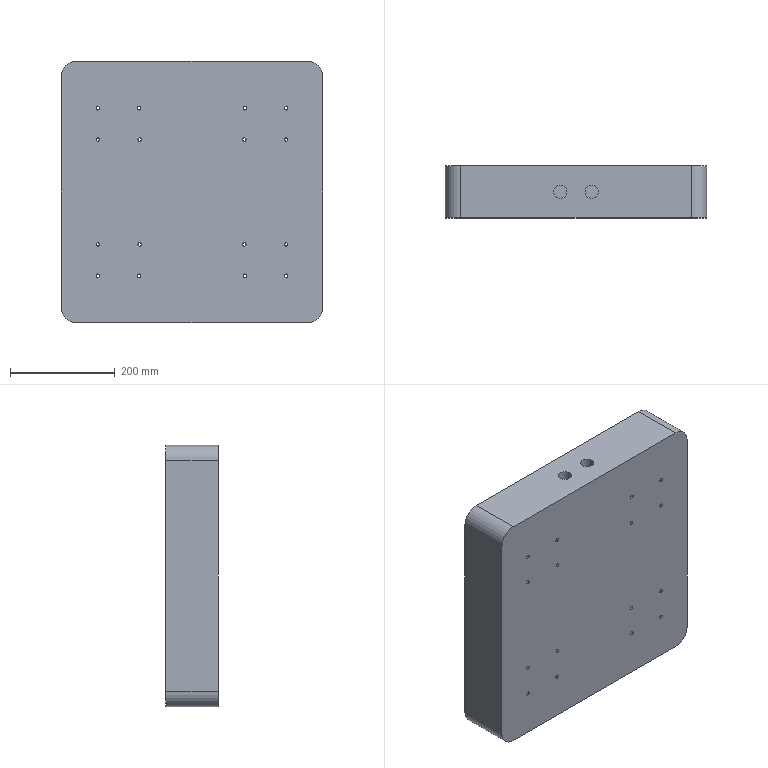Part | SolidWorks | features ICE 4, 3DProfileFeature 1, Extrusion 1, HoleWzd 1, MirrorPattern 1 | 1 solid | 145 faces | box 500 x 100 x 500 mm | volume 10401596 mm3 | cylinder 83 | cone 32 | plane 30 | commonest cylinder face diameters 6.6 x32 13 x32 50 x8 25 x4 60 x4 70 x3